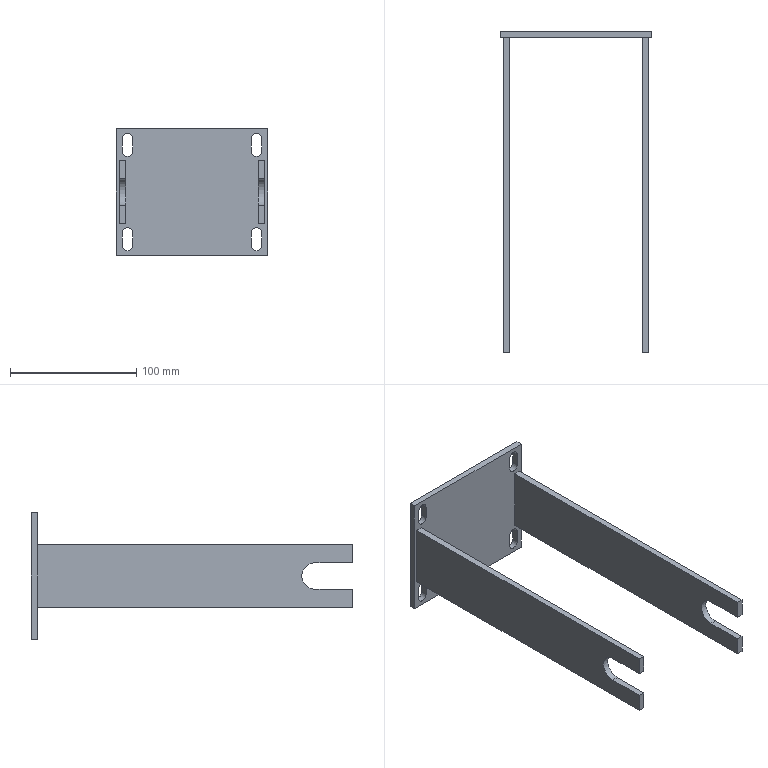Part | SolidWorks | features ICE 3, MirrorPattern 2, Extrusion 1 | 1 solid | 44 faces | box 120 x 255 x 100 mm | volume 174249 mm3 | plane 30 | cylinder 14 | commonest cylinder face diameters 8.258 x12 21 x2
STEP:
#1=CARTESIAN_POINT('',(111.116,0.,-3.551));
#2=VERTEX_POINT('',#1);
#3=CARTESIAN_POINT('',(115.245,0.,-7.68));
#4=VERTEX_POINT('',#3);
#5=CARTESIAN_POINT('',(111.116,0.,-7.68));
#6=DIRECTION('',(0.,1.,0.));
#7=DIRECTION('',(0.,0.,-1.));
#8=AXIS2_PLACEMENT_3D('',#5,#6,#7);
#9=CIRCLE('',#8,4.129);
#10=EDGE_CURVE('',#2,#4,#9,.T.);
#11=ORIENTED_EDGE('',*,*,#10,.F.);
#12=CARTESIAN_POINT('',(111.116,5.,-3.551));
#13=VERTEX_POINT('',#12);
#14=CARTESIAN_POINT('',(111.116,0.,-3.551));
#15=DIRECTION('',(0.,1.,0.));
#16=VECTOR('',#15,1000.);
#17=LINE('',#14,#16);
#18=EDGE_CURVE('',#2,#13,#17,.T.);
#19=ORIENTED_EDGE('',*,*,#18,.T.);
#20=CARTESIAN_POINT('',(115.245,5.,-7.68));
#21=VERTEX_POINT('',#20);
#22=CARTESIAN_POINT('',(111.116,5.,-7.68));
#23=DIRECTION('',(0.,1.,0.));
#24=DIRECTION('',(0.,0.,-1.));
#25=AXIS2_PLACEMENT_3D('',#22,#23,#24);
#26=CIRCLE('',#25,4.129);
#27=EDGE_CURVE('',#13,#21,#26,.T.);
#28=ORIENTED_EDGE('',*,*,#27,.T.);
#29=CARTESIAN_POINT('',(115.245,0.,-7.68));
#30=DIRECTION('',(0.,1.,0.));
#31=VECTOR('',#30,1000.);
#32=LINE('',#29,#31);
#33=EDGE_CURVE('',#4,#21,#32,.T.);
#34=ORIENTED_EDGE('',*,*,#33,.F.);
#35=EDGE_LOOP('',(#11,#19,#28,#34));
#36=FACE_OUTER_BOUND('',#35,.T.);
#37=CARTESIAN_POINT('',(111.116,0.,-7.68));
#38=DIRECTION('',(0.,1.,0.));
#39=DIRECTION('',(0.,0.,1.));
#40=AXIS2_PLACEMENT_3D('',#37,#38,#39);
#41=CYLINDRICAL_SURFACE('',#40,4.129);
#42=ADVANCED_FACE('',(#36),#41,.F.);
#43=CARTESIAN_POINT('',(13.013,0.,-7.68));
#44=VERTEX_POINT('',#43);
#45=CARTESIAN_POINT('',(8.884,0.,-3.551));
#46=VERTEX_POINT('',#45);
#47=CARTESIAN_POINT('',(8.884,0.,-7.68));
#48=DIRECTION('',(0.,-1.,0.));
#49=DIRECTION('',(0.,0.,-1.));
#50=AXIS2_PLACEMENT_3D('',#47,#48,#49);
#51=CIRCLE('',#50,4.129);
#52=EDGE_CURVE('',#44,#46,#51,.T.);
#53=ORIENTED_EDGE('',*,*,#52,.T.);
#54=CARTESIAN_POINT('',(8.884,5.,-3.551));
#55=VERTEX_POINT('',#54);
#56=CARTESIAN_POINT('',(8.884,0.,-3.551));
#57=DIRECTION('',(0.,1.,0.));
#58=VECTOR('',#57,1000.);
#59=LINE('',#56,#58);
#60=EDGE_CURVE('',#46,#55,#59,.T.);
#61=ORIENTED_EDGE('',*,*,#60,.T.);
#62=CARTESIAN_POINT('',(13.013,5.,-7.68));
#63=VERTEX_POINT('',#62);
#64=CARTESIAN_POINT('',(8.884,5.,-7.68));
#65=DIRECTION('',(0.,-1.,0.));
#66=DIRECTION('',(0.,0.,-1.));
#67=AXIS2_PLACEMENT_3D('',#64,#65,#66);
#68=CIRCLE('',#67,4.129);
#69=EDGE_CURVE('',#63,#55,#68,.T.);
#70=ORIENTED_EDGE('',*,*,#69,.F.);
#71=CARTESIAN_POINT('',(13.013,0.,-7.68));
#72=DIRECTION('',(0.,1.,0.));
#73=VECTOR('',#72,1000.);
#74=LINE('',#71,#73);
#75=EDGE_CURVE('',#44,#63,#74,.T.);
#76=ORIENTED_EDGE('',*,*,#75,.F.);
#77=EDGE_LOOP('',(#53,#61,#70,#76));
#78=FACE_OUTER_BOUND('',#77,.T.);
#79=CARTESIAN_POINT('',(8.884,0.,-7.68));
#80=DIRECTION('',(0.,1.,0.));
#81=DIRECTION('',(0.,0.,1.));
#82=AXIS2_PLACEMENT_3D('',#79,#80,#81);
#83=CYLINDRICAL_SURFACE('',#82,4.129);
#84=ADVANCED_FACE('',(#78),#83,.F.);
#85=CARTESIAN_POINT('',(115.245,0.,-82.342));
#86=VERTEX_POINT('',#85);
#87=CARTESIAN_POINT('',(111.116,0.,-78.214));
#88=VERTEX_POINT('',#87);
#89=CARTESIAN_POINT('',(111.116,0.,-82.342));
#90=DIRECTION('',(0.,-1.,0.));
#91=DIRECTION('',(0.,0.,1.));
#92=AXIS2_PLACEMENT_3D('',#89,#90,#91);
#93=CIRCLE('',#92,4.129);
#94=EDGE_CURVE('',#86,#88,#93,.T.);
#95=ORIENTED_EDGE('',*,*,#94,.T.);
#96=CARTESIAN_POINT('',(111.116,5.,-78.214));
#97=VERTEX_POINT('',#96);
#98=CARTESIAN_POINT('',(111.116,0.,-78.214));
#99=DIRECTION('',(0.,1.,0.));
#100=VECTOR('',#99,1000.);
#101=LINE('',#98,#100);
#102=EDGE_CURVE('',#88,#97,#101,.T.);
#103=ORIENTED_EDGE('',*,*,#102,.T.);
#104=CARTESIAN_POINT('',(115.245,5.,-82.342));
#105=VERTEX_POINT('',#104);
#106=CARTESIAN_POINT('',(111.116,5.,-82.342));
#107=DIRECTION('',(0.,-1.,0.));
#108=DIRECTION('',(0.,0.,1.));
#109=AXIS2_PLACEMENT_3D('',#106,#107,#108);
#110=CIRCLE('',#109,4.129);
#111=EDGE_CURVE('',#105,#97,#110,.T.);
#112=ORIENTED_EDGE('',*,*,#111,.F.);
#113=CARTESIAN_POINT('',(115.245,0.,-82.342));
#114=DIRECTION('',(0.,1.,0.));
#115=VECTOR('',#114,1000.);
#116=LINE('',#113,#115);
#117=EDGE_CURVE('',#86,#105,#116,.T.);
#118=ORIENTED_EDGE('',*,*,#117,.F.);
#119=EDGE_LOOP('',(#95,#103,#112,#118));
#120=FACE_OUTER_BOUND('',#119,.T.);
#121=CARTESIAN_POINT('',(111.116,0.,-82.342));
#122=DIRECTION('',(0.,1.,0.));
#123=DIRECTION('',(0.,0.,1.));
#124=AXIS2_PLACEMENT_3D('',#121,#122,#123);
#125=CYLINDRICAL_SURFACE('',#124,4.129);
#126=ADVANCED_FACE('',(#120),#125,.F.);
#127=CARTESIAN_POINT('',(8.884,0.,-78.214));
#128=VERTEX_POINT('',#127);
#129=CARTESIAN_POINT('',(13.013,0.,-82.342));
#130=VERTEX_POINT('',#129);
#131=CARTESIAN_POINT('',(8.884,0.,-82.342));
#132=DIRECTION('',(0.,1.,0.));
#133=DIRECTION('',(0.,0.,1.));
#134=AXIS2_PLACEMENT_3D('',#131,#132,#133);
#135=CIRCLE('',#134,4.129);
#136=EDGE_CURVE('',#128,#130,#135,.T.);
#137=ORIENTED_EDGE('',*,*,#136,.F.);
#138=CARTESIAN_POINT('',(8.884,5.,-78.214));
#139=VERTEX_POINT('',#138);
#140=CARTESIAN_POINT('',(8.884,0.,-78.214));
#141=DIRECTION('',(0.,1.,0.));
#142=VECTOR('',#141,1000.);
#143=LINE('',#140,#142);
#144=EDGE_CURVE('',#128,#139,#143,.T.);
#145=ORIENTED_EDGE('',*,*,#144,.T.);
#146=CARTESIAN_POINT('',(13.013,5.,-82.342));
#147=VERTEX_POINT('',#146);
#148=CARTESIAN_POINT('',(8.884,5.,-82.342));
#149=DIRECTION('',(0.,1.,0.));
#150=DIRECTION('',(0.,0.,1.));
#151=AXIS2_PLACEMENT_3D('',#148,#149,#150);
#152=CIRCLE('',#151,4.129);
#153=EDGE_CURVE('',#139,#147,#152,.T.);
#154=ORIENTED_EDGE('',*,*,#153,.T.);
#155=CARTESIAN_POINT('',(13.013,0.,-82.342));
#156=DIRECTION('',(0.,1.,0.));
#157=VECTOR('',#156,1000.);
#158=LINE('',#155,#157);
#159=EDGE_CURVE('',#130,#147,#158,.T.);
#160=ORIENTED_EDGE('',*,*,#159,.F.);
#161=EDGE_LOOP('',(#137,#145,#154,#160));
#162=FACE_OUTER_BOUND('',#161,.T.);
#163=CARTESIAN_POINT('',(8.884,0.,-82.342));
#164=DIRECTION('',(0.,1.,0.));
#165=DIRECTION('',(0.,0.,1.));
#166=AXIS2_PLACEMENT_3D('',#163,#164,#165);
#167=CYLINDRICAL_SURFACE('',#166,4.129);
#168=ADVANCED_FACE('',(#162),#167,.F.);
#169=CARTESIAN_POINT('',(117.5,-250.,-60.5));
#170=VERTEX_POINT('',#169);
#171=CARTESIAN_POINT('',(112.5,-250.,-60.5));
#172=VERTEX_POINT('',#171);
#173=CARTESIAN_POINT('',(452.5,-250.,-60.5));
#174=DIRECTION('',(-1.,0.,0.));
#175=VECTOR('',#174,1000.);
#176=LINE('',#173,#175);
#177=EDGE_CURVE('',#170,#172,#176,.T.);
#178=ORIENTED_EDGE('',*,*,#177,.T.);
#179=CARTESIAN_POINT('',(112.5,-250.,-75.));
#180=VERTEX_POINT('',#179);
#181=CARTESIAN_POINT('',(112.5,-250.,-45.));
#182=DIRECTION('',(0.,0.,-1.));
#183=VECTOR('',#182,1000.);
#184=LINE('',#181,#183);
#185=EDGE_CURVE('',#172,#180,#184,.T.);
#186=ORIENTED_EDGE('',*,*,#185,.T.);
#187=CARTESIAN_POINT('',(117.5,-250.,-75.));
#188=VERTEX_POINT('',#187);
#189=CARTESIAN_POINT('',(112.5,-250.,-75.));
#190=DIRECTION('',(1.,0.,0.));
#191=VECTOR('',#190,1000.);
#192=LINE('',#189,#191);
#193=EDGE_CURVE('',#180,#188,#192,.T.);
#194=ORIENTED_EDGE('',*,*,#193,.T.);
#195=CARTESIAN_POINT('',(117.5,-250.,-45.));
#196=DIRECTION('',(0.,0.,1.));
#197=VECTOR('',#196,1000.);
#198=LINE('',#195,#197);
#199=EDGE_CURVE('',#188,#170,#198,.T.);
#200=ORIENTED_EDGE('',*,*,#199,.T.);
#201=EDGE_LOOP('',(#178,#186,#194,#200));
#202=FACE_OUTER_BOUND('',#201,.T.);
#203=CARTESIAN_POINT('',(0.,-250.,0.));
#204=DIRECTION('',(0.,-1.,0.));
#205=DIRECTION('',(0.,0.,-1.));
#206=AXIS2_PLACEMENT_3D('',#203,#204,#205);
#207=PLANE('',#206);
#208=ADVANCED_FACE('',(#202),#207,.T.);
#209=CARTESIAN_POINT('',(7.5,-250.,-75.));
#210=VERTEX_POINT('',#209);
#211=CARTESIAN_POINT('',(7.5,-250.,-60.5));
#212=VERTEX_POINT('',#211);
#213=CARTESIAN_POINT('',(7.5,-250.,-50.));
#214=DIRECTION('',(0.,0.,1.));
#215=VECTOR('',#214,1000.);
#216=LINE('',#213,#215);
#217=EDGE_CURVE('',#210,#212,#216,.T.);
#218=ORIENTED_EDGE('',*,*,#217,.T.);
#219=CARTESIAN_POINT('',(2.5,-250.,-60.5));
#220=VERTEX_POINT('',#219);
#221=CARTESIAN_POINT('',(0.,-250.,-60.5));
#222=DIRECTION('',(-1.,0.,0.));
#223=VECTOR('',#222,1000.);
#224=LINE('',#221,#223);
#225=EDGE_CURVE('',#212,#220,#224,.T.);
#226=ORIENTED_EDGE('',*,*,#225,.T.);
#227=CARTESIAN_POINT('',(2.5,-250.,-75.));
#228=VERTEX_POINT('',#227);
#229=CARTESIAN_POINT('',(2.5,-250.,-50.));
#230=DIRECTION('',(0.,0.,-1.));
#231=VECTOR('',#230,1000.);
#232=LINE('',#229,#231);
#233=EDGE_CURVE('',#220,#228,#232,.T.);
#234=ORIENTED_EDGE('',*,*,#233,.T.);
#235=CARTESIAN_POINT('',(7.5,-250.,-75.));
#236=DIRECTION('',(1.,0.,0.));
#237=VECTOR('',#236,1000.);
#238=LINE('',#235,#237);
#239=EDGE_CURVE('',#228,#210,#238,.T.);
#240=ORIENTED_EDGE('',*,*,#239,.T.);
#241=EDGE_LOOP('',(#218,#226,#234,#240));
#242=FACE_OUTER_BOUND('',#241,.T.);
#243=CARTESIAN_POINT('',(0.,-250.,0.));
#244=DIRECTION('',(0.,1.,0.));
#245=DIRECTION('',(0.,0.,1.));
#246=AXIS2_PLACEMENT_3D('',#243,#244,#245);
#247=PLANE('',#246);
#248=ADVANCED_FACE('',(#242),#247,.F.);
#249=CARTESIAN_POINT('',(112.5,0.,-75.));
#250=VERTEX_POINT('',#249);
#251=CARTESIAN_POINT('',(117.5,0.,-75.));
#252=VERTEX_POINT('',#251);
#253=CARTESIAN_POINT('',(112.5,0.,-75.));
#254=DIRECTION('',(1.,0.,0.));
#255=VECTOR('',#254,1000.);
#256=LINE('',#253,#255);
#257=EDGE_CURVE('',#250,#252,#256,.T.);
#258=ORIENTED_EDGE('',*,*,#257,.F.);
#259=CARTESIAN_POINT('',(112.5,0.,-25.));
#260=VERTEX_POINT('',#259);
#261=CARTESIAN_POINT('',(112.5,0.,-45.));
#262=DIRECTION('',(0.,0.,-1.));
#263=VECTOR('',#262,1000.);
#264=LINE('',#261,#263);
#265=EDGE_CURVE('',#260,#250,#264,.T.);
#266=ORIENTED_EDGE('',*,*,#265,.F.);
#267=CARTESIAN_POINT('',(117.5,0.,-25.));
#268=VERTEX_POINT('',#267);
#269=CARTESIAN_POINT('',(117.5,0.,-25.));
#270=DIRECTION('',(-1.,0.,0.));
#271=VECTOR('',#270,1000.);
#272=LINE('',#269,#271);
#273=EDGE_CURVE('',#268,#260,#272,.T.);
#274=ORIENTED_EDGE('',*,*,#273,.F.);
#275=CARTESIAN_POINT('',(117.5,0.,-45.));
#276=DIRECTION('',(0.,0.,1.));
#277=VECTOR('',#276,1000.);
#278=LINE('',#275,#277);
#279=EDGE_CURVE('',#252,#268,#278,.T.);
#280=ORIENTED_EDGE('',*,*,#279,.F.);
#281=EDGE_LOOP('',(#258,#266,#274,#280));
#282=FACE_BOUND('',#281,.T.);
#283=CARTESIAN_POINT('',(106.987,0.,-7.68));
#284=VERTEX_POINT('',#283);
#285=CARTESIAN_POINT('',(111.116,0.,-7.68));
#286=DIRECTION('',(0.,1.,0.));
#287=DIRECTION('',(0.,0.,-1.));
#288=AXIS2_PLACEMENT_3D('',#285,#286,#287);
#289=CIRCLE('',#288,4.129);
#290=EDGE_CURVE('',#284,#2,#289,.T.);
#291=ORIENTED_EDGE('',*,*,#290,.T.);
#292=ORIENTED_EDGE('',*,*,#10,.T.);
#293=CARTESIAN_POINT('',(115.245,0.,-17.658));
#294=VERTEX_POINT('',#293);
#295=CARTESIAN_POINT('',(115.245,0.,-7.68));
#296=DIRECTION('',(0.,0.,-1.));
#297=VECTOR('',#296,1000.);
#298=LINE('',#295,#297);
#299=EDGE_CURVE('',#4,#294,#298,.T.);
#300=ORIENTED_EDGE('',*,*,#299,.T.);
#301=CARTESIAN_POINT('',(106.987,0.,-17.658));
#302=VERTEX_POINT('',#301);
#303=CARTESIAN_POINT('',(111.116,0.,-17.658));
#304=DIRECTION('',(0.,1.,0.));
#305=DIRECTION('',(0.,0.,-1.));
#306=AXIS2_PLACEMENT_3D('',#303,#304,#305);
#307=CIRCLE('',#306,4.129);
#308=EDGE_CURVE('',#294,#302,#307,.T.);
#309=ORIENTED_EDGE('',*,*,#308,.T.);
#310=CARTESIAN_POINT('',(106.987,0.,-7.68));
#311=DIRECTION('',(0.,0.,1.));
#312=VECTOR('',#311,1000.);
#313=LINE('',#310,#312);
#314=EDGE_CURVE('',#302,#284,#313,.T.);
#315=ORIENTED_EDGE('',*,*,#314,.T.);
#316=EDGE_LOOP('',(#291,#292,#300,#309,#315));
#317=FACE_BOUND('',#316,.T.);
#318=CARTESIAN_POINT('',(115.245,0.,-92.32));
#319=VERTEX_POINT('',#318);
#320=CARTESIAN_POINT('',(115.245,0.,-92.32));
#321=DIRECTION('',(0.,0.,1.));
#322=VECTOR('',#321,1000.);
#323=LINE('',#320,#322);
#324=EDGE_CURVE('',#319,#86,#323,.T.);
#325=ORIENTED_EDGE('',*,*,#324,.F.);
#326=CARTESIAN_POINT('',(106.987,0.,-92.32));
#327=VERTEX_POINT('',#326);
#328=CARTESIAN_POINT('',(111.116,0.,-92.32));
#329=DIRECTION('',(0.,-1.,0.));
#330=DIRECTION('',(0.,0.,1.));
#331=AXIS2_PLACEMENT_3D('',#328,#329,#330);
#332=CIRCLE('',#331,4.129);
#333=EDGE_CURVE('',#327,#319,#332,.T.);
#334=ORIENTED_EDGE('',*,*,#333,.F.);
#335=CARTESIAN_POINT('',(106.987,0.,-82.342));
#336=VERTEX_POINT('',#335);
#337=CARTESIAN_POINT('',(106.987,0.,-92.32));
#338=DIRECTION('',(0.,0.,-1.));
#339=VECTOR('',#338,1000.);
#340=LINE('',#337,#339);
#341=EDGE_CURVE('',#336,#327,#340,.T.);
#342=ORIENTED_EDGE('',*,*,#341,.F.);
#343=CARTESIAN_POINT('',(111.116,0.,-82.342));
#344=DIRECTION('',(0.,-1.,0.));
#345=DIRECTION('',(0.,0.,1.));
#346=AXIS2_PLACEMENT_3D('',#343,#344,#345);
#347=CIRCLE('',#346,4.129);
#348=EDGE_CURVE('',#88,#336,#347,.T.);
#349=ORIENTED_EDGE('',*,*,#348,.F.);
#350=ORIENTED_EDGE('',*,*,#94,.F.);
#351=EDGE_LOOP('',(#325,#334,#342,#349,#350));
#352=FACE_BOUND('',#351,.T.);
#353=CARTESIAN_POINT('',(13.013,0.,-92.32));
#354=VERTEX_POINT('',#353);
#355=CARTESIAN_POINT('',(4.755,0.,-92.32));
#356=VERTEX_POINT('',#355);
#357=CARTESIAN_POINT('',(8.884,0.,-92.32));
#358=DIRECTION('',(0.,1.,0.));
#359=DIRECTION('',(0.,0.,1.));
#360=AXIS2_PLACEMENT_3D('',#357,#358,#359);
#361=CIRCLE('',#360,4.129);
#362=EDGE_CURVE('',#354,#356,#361,.T.);
#363=ORIENTED_EDGE('',*,*,#362,.T.);
#364=CARTESIAN_POINT('',(4.755,0.,-82.342));
#365=VERTEX_POINT('',#364);
#366=CARTESIAN_POINT('',(4.755,0.,-92.32));
#367=DIRECTION('',(0.,0.,1.));
#368=VECTOR('',#367,1000.);
#369=LINE('',#366,#368);
#370=EDGE_CURVE('',#356,#365,#369,.T.);
#371=ORIENTED_EDGE('',*,*,#370,.T.);
#372=CARTESIAN_POINT('',(8.884,0.,-82.342));
#373=DIRECTION('',(0.,1.,0.));
#374=DIRECTION('',(0.,0.,1.));
#375=AXIS2_PLACEMENT_3D('',#372,#373,#374);
#376=CIRCLE('',#375,4.129);
#377=EDGE_CURVE('',#365,#128,#376,.T.);
#378=ORIENTED_EDGE('',*,*,#377,.T.);
#379=ORIENTED_EDGE('',*,*,#136,.T.);
#380=CARTESIAN_POINT('',(13.013,0.,-92.32));
#381=DIRECTION('',(0.,0.,-1.));
#382=VECTOR('',#381,1000.);
#383=LINE('',#380,#382);
#384=EDGE_CURVE('',#130,#354,#383,.T.);
#385=ORIENTED_EDGE('',*,*,#384,.T.);
#386=EDGE_LOOP('',(#363,#371,#378,#379,#385));
#387=FACE_BOUND('',#386,.T.);
#388=CARTESIAN_POINT('',(0.,0.,-100.));
#389=VERTEX_POINT('',#388);
#390=CARTESIAN_POINT('',(0.,0.,0.));
#391=VERTEX_POINT('',#390);
#392=CARTESIAN_POINT('',(0.,0.,0.));
#393=DIRECTION('',(0.,0.,1.));
#394=VECTOR('',#393,1000.);
#395=LINE('',#392,#394);
#396=EDGE_CURVE('',#389,#391,#395,.T.);
#397=ORIENTED_EDGE('',*,*,#396,.F.);
#398=CARTESIAN_POINT('',(120.,0.,-100.));
#399=VERTEX_POINT('',#398);
#400=CARTESIAN_POINT('',(0.,0.,-100.));
#401=DIRECTION('',(-1.,0.,0.));
#402=VECTOR('',#401,1000.);
#403=LINE('',#400,#402);
#404=EDGE_CURVE('',#399,#389,#403,.T.);
#405=ORIENTED_EDGE('',*,*,#404,.F.);
#406=CARTESIAN_POINT('',(120.,0.,0.));
#407=VERTEX_POINT('',#406);
#408=CARTESIAN_POINT('',(120.,0.,0.));
#409=DIRECTION('',(0.,0.,-1.));
#410=VECTOR('',#409,1000.);
#411=LINE('',#408,#410);
#412=EDGE_CURVE('',#407,#399,#411,.T.);
#413=ORIENTED_EDGE('',*,*,#412,.F.);
#414=CARTESIAN_POINT('',(0.,0.,0.));
#415=DIRECTION('',(1.,0.,0.));
#416=VECTOR('',#415,1000.);
#417=LINE('',#414,#416);
#418=EDGE_CURVE('',#391,#407,#417,.T.);
#419=ORIENTED_EDGE('',*,*,#418,.F.);
#420=EDGE_LOOP('',(#397,#405,#413,#419));
#421=FACE_OUTER_BOUND('',#420,.T.);
#422=CARTESIAN_POINT('',(4.755,0.,-7.68));
#423=VERTEX_POINT('',#422);
#424=CARTESIAN_POINT('',(4.755,0.,-17.658));
#425=VERTEX_POINT('',#424);
#426=CARTESIAN_POINT('',(4.755,0.,-7.68));
#427=DIRECTION('',(0.,0.,-1.));
#428=VECTOR('',#427,1000.);
#429=LINE('',#426,#428);
#430=EDGE_CURVE('',#423,#425,#429,.T.);
#431=ORIENTED_EDGE('',*,*,#430,.F.);
#432=CARTESIAN_POINT('',(8.884,0.,-7.68));
#433=DIRECTION('',(0.,-1.,0.));
#434=DIRECTION('',(0.,0.,-1.));
#435=AXIS2_PLACEMENT_3D('',#432,#433,#434);
#436=CIRCLE('',#435,4.129);
#437=EDGE_CURVE('',#46,#423,#436,.T.);
#438=ORIENTED_EDGE('',*,*,#437,.F.);
#439=ORIENTED_EDGE('',*,*,#52,.F.);
#440=CARTESIAN_POINT('',(13.013,0.,-17.658));
#441=VERTEX_POINT('',#440);
#442=CARTESIAN_POINT('',(13.013,0.,-7.68));
#443=DIRECTION('',(0.,0.,1.));
#444=VECTOR('',#443,1000.);
#445=LINE('',#442,#444);
#446=EDGE_CURVE('',#441,#44,#445,.T.);
#447=ORIENTED_EDGE('',*,*,#446,.F.);
#448=CARTESIAN_POINT('',(8.884,0.,-17.658));
#449=DIRECTION('',(0.,-1.,0.));
#450=DIRECTION('',(0.,0.,-1.));
#451=AXIS2_PLACEMENT_3D('',#448,#449,#450);
#452=CIRCLE('',#451,4.129);
#453=EDGE_CURVE('',#425,#441,#452,.T.);
#454=ORIENTED_EDGE('',*,*,#453,.F.);
#455=EDGE_LOOP('',(#431,#438,#439,#447,#454));
#456=FACE_BOUND('',#455,.T.);
#457=CARTESIAN_POINT('',(2.5,0.,-75.));
#458=VERTEX_POINT('',#457);
#459=CARTESIAN_POINT('',(7.5,0.,-75.));
#460=VERTEX_POINT('',#459);
#461=CARTESIAN_POINT('',(7.5,0.,-75.));
#462=DIRECTION('',(1.,0.,0.));
#463=VECTOR('',#462,1000.);
#464=LINE('',#461,#463);
#465=EDGE_CURVE('',#458,#460,#464,.T.);
#466=ORIENTED_EDGE('',*,*,#465,.F.);
#467=CARTESIAN_POINT('',(2.5,0.,-25.));
#468=VERTEX_POINT('',#467);
#469=CARTESIAN_POINT('',(2.5,0.,-50.));
#470=DIRECTION('',(0.,0.,-1.));
#471=VECTOR('',#470,1000.);
#472=LINE('',#469,#471);
#473=EDGE_CURVE('',#468,#458,#472,.T.);
#474=ORIENTED_EDGE('',*,*,#473,.F.);
#475=CARTESIAN_POINT('',(7.5,0.,-25.));
#476=VERTEX_POINT('',#475);
#477=CARTESIAN_POINT('',(2.5,0.,-25.));
#478=DIRECTION('',(-1.,0.,0.));
#479=VECTOR('',#478,1000.);
#480=LINE('',#477,#479);
#481=EDGE_CURVE('',#476,#468,#480,.T.);
#482=ORIENTED_EDGE('',*,*,#481,.F.);
#483=CARTESIAN_POINT('',(7.5,0.,-50.));
#484=DIRECTION('',(0.,0.,1.));
#485=VECTOR('',#484,1000.);
#486=LINE('',#483,#485);
#487=EDGE_CURVE('',#460,#476,#486,.T.);
#488=ORIENTED_EDGE('',*,*,#487,.F.);
#489=EDGE_LOOP('',(#466,#474,#482,#488));
#490=FACE_BOUND('',#489,.T.);
#491=CARTESIAN_POINT('',(0.,0.,0.));
#492=DIRECTION('',(0.,-1.,0.));
#493=DIRECTION('',(0.,0.,-1.));
#494=AXIS2_PLACEMENT_3D('',#491,#492,#493);
#495=PLANE('',#494);
#496=ADVANCED_FACE('',(#282,#317,#352,#387,#421,#456,#490),#495,.T.);
#497=CARTESIAN_POINT('',(115.245,5.,-17.658));
#498=VERTEX_POINT('',#497);
#499=CARTESIAN_POINT('',(115.245,5.,-7.68));
#500=DIRECTION('',(0.,0.,-1.));
#501=VECTOR('',#500,1000.);
#502=LINE('',#499,#501);
#503=EDGE_CURVE('',#21,#498,#502,.T.);
#504=ORIENTED_EDGE('',*,*,#503,.F.);
#505=ORIENTED_EDGE('',*,*,#27,.F.);
#506=CARTESIAN_POINT('',(106.987,5.,-7.68));
#507=VERTEX_POINT('',#506);
#508=CARTESIAN_POINT('',(111.116,5.,-7.68));
#509=DIRECTION('',(0.,1.,0.));
#510=DIRECTION('',(0.,0.,-1.));
#511=AXIS2_PLACEMENT_3D('',#508,#509,#510);
#512=CIRCLE('',#511,4.129);
#513=EDGE_CURVE('',#507,#13,#512,.T.);
#514=ORIENTED_EDGE('',*,*,#513,.F.);
#515=CARTESIAN_POINT('',(106.987,5.,-17.658));
#516=VERTEX_POINT('',#515);
#517=CARTESIAN_POINT('',(106.987,5.,-7.68));
#518=DIRECTION('',(0.,0.,1.));
#519=VECTOR('',#518,1000.);
#520=LINE('',#517,#519);
#521=EDGE_CURVE('',#516,#507,#520,.T.);
#522=ORIENTED_EDGE('',*,*,#521,.F.);
#523=CARTESIAN_POINT('',(111.116,5.,-17.658));
#524=DIRECTION('',(0.,1.,0.));
#525=DIRECTION('',(0.,0.,-1.));
#526=AXIS2_PLACEMENT_3D('',#523,#524,#525);
#527=CIRCLE('',#526,4.129);
#528=EDGE_CURVE('',#498,#516,#527,.T.);
#529=ORIENTED_EDGE('',*,*,#528,.F.);
#530=EDGE_LOOP('',(#504,#505,#514,#522,#529));
#531=FACE_BOUND('',#530,.T.);
#532=CARTESIAN_POINT('',(106.987,5.,-92.32));
#533=VERTEX_POINT('',#532);
#534=CARTESIAN_POINT('',(115.245,5.,-92.32));
#535=VERTEX_POINT('',#534);
#536=CARTESIAN_POINT('',(111.116,5.,-92.32));
#537=DIRECTION('',(0.,-1.,0.));
#538=DIRECTION('',(0.,0.,1.));
#539=AXIS2_PLACEMENT_3D('',#536,#537,#538);
#540=CIRCLE('',#539,4.129);
#541=EDGE_CURVE('',#533,#535,#540,.T.);
#542=ORIENTED_EDGE('',*,*,#541,.T.);
#543=CARTESIAN_POINT('',(115.245,5.,-92.32));
#544=DIRECTION('',(0.,0.,1.));
#545=VECTOR('',#544,1000.);
#546=LINE('',#543,#545);
#547=EDGE_CURVE('',#535,#105,#546,.T.);
#548=ORIENTED_EDGE('',*,*,#547,.T.);
#549=ORIENTED_EDGE('',*,*,#111,.T.);
#550=CARTESIAN_POINT('',(106.987,5.,-82.342));
#551=VERTEX_POINT('',#550);
#552=CARTESIAN_POINT('',(111.116,5.,-82.342));
#553=DIRECTION('',(0.,-1.,0.));
#554=DIRECTION('',(0.,0.,1.));
#555=AXIS2_PLACEMENT_3D('',#552,#553,#554);
#556=CIRCLE('',#555,4.129);
#557=EDGE_CURVE('',#97,#551,#556,.T.);
#558=ORIENTED_EDGE('',*,*,#557,.T.);
#559=CARTESIAN_POINT('',(106.987,5.,-92.32));
#560=DIRECTION('',(0.,0.,-1.));
#561=VECTOR('',#560,1000.);
#562=LINE('',#559,#561);
#563=EDGE_CURVE('',#551,#533,#562,.T.);
#564=ORIENTED_EDGE('',*,*,#563,.T.);
#565=EDGE_LOOP('',(#542,#548,#549,#558,#564));
#566=FACE_BOUND('',#565,.T.);
#567=CARTESIAN_POINT('',(4.755,5.,-92.32));
#568=VERTEX_POINT('',#567);
#569=CARTESIAN_POINT('',(4.755,5.,-82.342));
#570=VERTEX_POINT('',#569);
#571=CARTESIAN_POINT('',(4.755,5.,-92.32));
#572=DIRECTION('',(0.,0.,1.));
#573=VECTOR('',#572,1000.);
#574=LINE('',#571,#573);
#575=EDGE_CURVE('',#568,#570,#574,.T.);
#576=ORIENTED_EDGE('',*,*,#575,.F.);
#577=CARTESIAN_POINT('',(13.013,5.,-92.32));
#578=VERTEX_POINT('',#577);
#579=CARTESIAN_POINT('',(8.884,5.,-92.32));
#580=DIRECTION('',(0.,1.,0.));
#581=DIRECTION('',(0.,0.,1.));
#582=AXIS2_PLACEMENT_3D('',#579,#580,#581);
#583=CIRCLE('',#582,4.129);
#584=EDGE_CURVE('',#578,#568,#583,.T.);
#585=ORIENTED_EDGE('',*,*,#584,.F.);
#586=CARTESIAN_POINT('',(13.013,5.,-92.32));
#587=DIRECTION('',(0.,0.,-1.));
#588=VECTOR('',#587,1000.);
#589=LINE('',#586,#588);
#590=EDGE_CURVE('',#147,#578,#589,.T.);
#591=ORIENTED_EDGE('',*,*,#590,.F.);
#592=ORIENTED_EDGE('',*,*,#153,.F.);
#593=CARTESIAN_POINT('',(8.884,5.,-82.342));
#594=DIRECTION('',(0.,1.,0.));
#595=DIRECTION('',(0.,0.,1.));
#596=AXIS2_PLACEMENT_3D('',#593,#594,#595);
#597=CIRCLE('',#596,4.129);
#598=EDGE_CURVE('',#570,#139,#597,.T.);
#599=ORIENTED_EDGE('',*,*,#598,.F.);
#600=EDGE_LOOP('',(#576,#585,#591,#592,#599));
#601=FACE_BOUND('',#600,.T.);
#602=CARTESIAN_POINT('',(0.,5.,-100.));
#603=VERTEX_POINT('',#602);
#604=CARTESIAN_POINT('',(0.,5.,0.));
#605=VERTEX_POINT('',#604);
#606=CARTESIAN_POINT('',(0.,5.,0.));
#607=DIRECTION('',(0.,0.,1.));
#608=VECTOR('',#607,1000.);
#609=LINE('',#606,#608);
#610=EDGE_CURVE('',#603,#605,#609,.T.);
#611=ORIENTED_EDGE('',*,*,#610,.T.);
#612=CARTESIAN_POINT('',(120.,5.,0.));
#613=VERTEX_POINT('',#612);
#614=CARTESIAN_POINT('',(0.,5.,0.));
#615=DIRECTION('',(1.,0.,0.));
#616=VECTOR('',#615,1000.);
#617=LINE('',#614,#616);
#618=EDGE_CURVE('',#605,#613,#617,.T.);
#619=ORIENTED_EDGE('',*,*,#618,.T.);
#620=CARTESIAN_POINT('',(120.,5.,-100.));
#621=VERTEX_POINT('',#620);
#622=CARTESIAN_POINT('',(120.,5.,0.));
#623=DIRECTION('',(0.,0.,-1.));
#624=VECTOR('',#623,1000.);
#625=LINE('',#622,#624);
#626=EDGE_CURVE('',#613,#621,#625,.T.);
#627=ORIENTED_EDGE('',*,*,#626,.T.);
#628=CARTESIAN_POINT('',(0.,5.,-100.));
#629=DIRECTION('',(-1.,0.,0.));
#630=VECTOR('',#629,1000.);
#631=LINE('',#628,#630);
#632=EDGE_CURVE('',#621,#603,#631,.T.);
#633=ORIENTED_EDGE('',*,*,#632,.T.);
#634=EDGE_LOOP('',(#611,#619,#627,#633));
#635=FACE_OUTER_BOUND('',#634,.T.);
#636=ORIENTED_EDGE('',*,*,#69,.T.);
#637=CARTESIAN_POINT('',(4.755,5.,-7.68));
#638=VERTEX_POINT('',#637);
#639=CARTESIAN_POINT('',(8.884,5.,-7.68));
#640=DIRECTION('',(0.,-1.,0.));
#641=DIRECTION('',(0.,0.,-1.));
#642=AXIS2_PLACEMENT_3D('',#639,#640,#641);
#643=CIRCLE('',#642,4.129);
#644=EDGE_CURVE('',#55,#638,#643,.T.);
#645=ORIENTED_EDGE('',*,*,#644,.T.);
#646=CARTESIAN_POINT('',(4.755,5.,-17.658));
#647=VERTEX_POINT('',#646);
#648=CARTESIAN_POINT('',(4.755,5.,-7.68));
#649=DIRECTION('',(0.,0.,-1.));
#650=VECTOR('',#649,1000.);
#651=LINE('',#648,#650);
#652=EDGE_CURVE('',#638,#647,#651,.T.);
#653=ORIENTED_EDGE('',*,*,#652,.T.);
#654=CARTESIAN_POINT('',(13.013,5.,-17.658));
#655=VERTEX_POINT('',#654);
#656=CARTESIAN_POINT('',(8.884,5.,-17.658));
#657=DIRECTION('',(0.,-1.,0.));
#658=DIRECTION('',(0.,0.,-1.));
#659=AXIS2_PLACEMENT_3D('',#656,#657,#658);
#660=CIRCLE('',#659,4.129);
#661=EDGE_CURVE('',#647,#655,#660,.T.);
#662=ORIENTED_EDGE('',*,*,#661,.T.);
#663=CARTESIAN_POINT('',(13.013,5.,-7.68));
#664=DIRECTION('',(0.,0.,1.));
#665=VECTOR('',#664,1000.);
#666=LINE('',#663,#665);
#667=EDGE_CURVE('',#655,#63,#666,.T.);
#668=ORIENTED_EDGE('',*,*,#667,.T.);
#669=EDGE_LOOP('',(#636,#645,#653,#662,#668));
#670=FACE_BOUND('',#669,.T.);
#671=CARTESIAN_POINT('',(0.,5.,0.));
#672=DIRECTION('',(0.,-1.,0.));
#673=DIRECTION('',(0.,0.,-1.));
#674=AXIS2_PLACEMENT_3D('',#671,#672,#673);
#675=PLANE('',#674);
#676=ADVANCED_FACE('',(#531,#566,#601,#635,#670),#675,.F.);
#677=ORIENTED_EDGE('',*,*,#396,.T.);
#678=CARTESIAN_POINT('',(0.,5.,0.));
#679=DIRECTION('',(0.,-1.,0.));
#680=VECTOR('',#679,1000.);
#681=LINE('',#678,#680);
#682=EDGE_CURVE('',#605,#391,#681,.T.);
#683=ORIENTED_EDGE('',*,*,#682,.F.);
#684=ORIENTED_EDGE('',*,*,#610,.F.);
#685=CARTESIAN_POINT('',(0.,5.,-100.));
#686=DIRECTION('',(0.,-1.,0.));
#687=VECTOR('',#686,1000.);
#688=LINE('',#685,#687);
#689=EDGE_CURVE('',#603,#389,#688,.T.);
#690=ORIENTED_EDGE('',*,*,#689,.T.);
#691=EDGE_LOOP('',(#677,#683,#684,#690));
#692=FACE_OUTER_BOUND('',#691,.T.);
#693=CARTESIAN_POINT('',(0.,5.,0.));
#694=DIRECTION('',(1.,0.,0.));
#695=DIRECTION('',(0.,0.,-1.));
#696=AXIS2_PLACEMENT_3D('',#693,#694,#695);
#697=PLANE('',#696);
#698=ADVANCED_FACE('',(#692),#697,.F.);
#699=ORIENTED_EDGE('',*,*,#418,.T.);
#700=CARTESIAN_POINT('',(120.,5.,0.));
#701=DIRECTION('',(0.,-1.,0.));
#702=VECTOR('',#701,1000.);
#703=LINE('',#700,#702);
#704=EDGE_CURVE('',#613,#407,#703,.T.);
#705=ORIENTED_EDGE('',*,*,#704,.F.);
#706=ORIENTED_EDGE('',*,*,#618,.F.);
#707=ORIENTED_EDGE('',*,*,#682,.T.);
#708=EDGE_LOOP('',(#699,#705,#706,#707));
#709=FACE_OUTER_BOUND('',#708,.T.);
#710=CARTESIAN_POINT('',(0.,5.,0.));
#711=DIRECTION('',(0.,0.,-1.));
#712=DIRECTION('',(-1.,0.,0.));
#713=AXIS2_PLACEMENT_3D('',#710,#711,#712);
#714=PLANE('',#713);
#715=ADVANCED_FACE('',(#709),#714,.F.);
#716=ORIENTED_EDGE('',*,*,#412,.T.);
#717=CARTESIAN_POINT('',(120.,5.,-100.));
#718=DIRECTION('',(0.,-1.,0.));
#719=VECTOR('',#718,1000.);
#720=LINE('',#717,#719);
#721=EDGE_CURVE('',#621,#399,#720,.T.);
#722=ORIENTED_EDGE('',*,*,#721,.F.);
#723=ORIENTED_EDGE('',*,*,#626,.F.);
#724=ORIENTED_EDGE('',*,*,#704,.T.);
#725=EDGE_LOOP('',(#716,#722,#723,#724));
#726=FACE_OUTER_BOUND('',#725,.T.);
#727=CARTESIAN_POINT('',(120.,5.,0.));
#728=DIRECTION('',(-1.,0.,0.));
#729=DIRECTION('',(0.,0.,1.));
#730=AXIS2_PLACEMENT_3D('',#727,#728,#729);
#731=PLANE('',#730);
#732=ADVANCED_FACE('',(#726),#731,.F.);
#733=ORIENTED_EDGE('',*,*,#404,.T.);
#734=ORIENTED_EDGE('',*,*,#689,.F.);
#735=ORIENTED_EDGE('',*,*,#632,.F.);
#736=ORIENTED_EDGE('',*,*,#721,.T.);
#737=EDGE_LOOP('',(#733,#734,#735,#736));
#738=FACE_OUTER_BOUND('',#737,.T.);
#739=CARTESIAN_POINT('',(0.,5.,-100.));
#740=DIRECTION('',(0.,0.,1.));
#741=DIRECTION('',(1.,0.,0.));
#742=AXIS2_PLACEMENT_3D('',#739,#740,#741);
#743=PLANE('',#742);
#744=ADVANCED_FACE('',(#738),#743,.F.);
#745=ORIENTED_EDGE('',*,*,#584,.T.);
#746=CARTESIAN_POINT('',(4.755,0.,-92.32));
#747=DIRECTION('',(0.,1.,0.));
#748=VECTOR('',#747,1000.);
#749=LINE('',#746,#748);
#750=EDGE_CURVE('',#356,#568,#749,.T.);
#751=ORIENTED_EDGE('',*,*,#750,.F.);
#752=ORIENTED_EDGE('',*,*,#362,.F.);
#753=CARTESIAN_POINT('',(13.013,0.,-92.32));
#754=DIRECTION('',(0.,1.,0.));
#755=VECTOR('',#754,1000.);
#756=LINE('',#753,#755);
#757=EDGE_CURVE('',#354,#578,#756,.T.);
#758=ORIENTED_EDGE('',*,*,#757,.T.);
#759=EDGE_LOOP('',(#745,#751,#752,#758));
#760=FACE_OUTER_BOUND('',#759,.T.);
#761=CARTESIAN_POINT('',(8.884,0.,-92.32));
#762=DIRECTION('',(0.,1.,0.));
#763=DIRECTION('',(0.,0.,1.));
#764=AXIS2_PLACEMENT_3D('',#761,#762,#763);
#765=CYLINDRICAL_SURFACE('',#764,4.129);
#766=ADVANCED_FACE('',(#760),#765,.F.);
#767=ORIENTED_EDGE('',*,*,#590,.T.);
#768=ORIENTED_EDGE('',*,*,#757,.F.);
#769=ORIENTED_EDGE('',*,*,#384,.F.);
#770=ORIENTED_EDGE('',*,*,#159,.T.);
#771=EDGE_LOOP('',(#767,#768,#769,#770));
#772=FACE_OUTER_BOUND('',#771,.T.);
#773=CARTESIAN_POINT('',(13.013,0.,-92.32));
#774=DIRECTION('',(1.,0.,0.));
#775=DIRECTION('',(0.,0.,-1.));
#776=AXIS2_PLACEMENT_3D('',#773,#774,#775);
#777=PLANE('',#776);
#778=ADVANCED_FACE('',(#772),#777,.F.);
#779=ORIENTED_EDGE('',*,*,#144,.F.);
#780=ORIENTED_EDGE('',*,*,#377,.F.);
#781=CARTESIAN_POINT('',(4.755,0.,-82.342));
#782=DIRECTION('',(0.,1.,0.));
#783=VECTOR('',#782,1000.);
#784=LINE('',#781,#783);
#785=EDGE_CURVE('',#365,#570,#784,.T.);
#786=ORIENTED_EDGE('',*,*,#785,.T.);
#787=ORIENTED_EDGE('',*,*,#598,.T.);
#788=EDGE_LOOP('',(#779,#780,#786,#787));
#789=FACE_OUTER_BOUND('',#788,.T.);
#790=CARTESIAN_POINT('',(8.884,0.,-82.342));
#791=DIRECTION('',(0.,1.,0.));
#792=DIRECTION('',(0.,0.,1.));
#793=AXIS2_PLACEMENT_3D('',#790,#791,#792);
#794=CYLINDRICAL_SURFACE('',#793,4.129);
#795=ADVANCED_FACE('',(#789),#794,.F.);
#796=ORIENTED_EDGE('',*,*,#575,.T.);
#797=ORIENTED_EDGE('',*,*,#785,.F.);
#798=ORIENTED_EDGE('',*,*,#370,.F.);
#799=ORIENTED_EDGE('',*,*,#750,.T.);
#800=EDGE_LOOP('',(#796,#797,#798,#799));
#801=FACE_OUTER_BOUND('',#800,.T.);
#802=CARTESIAN_POINT('',(4.755,0.,-92.32));
#803=DIRECTION('',(-1.,0.,0.));
#804=DIRECTION('',(0.,0.,1.));
#805=AXIS2_PLACEMENT_3D('',#802,#803,#804);
#806=PLANE('',#805);
#807=ADVANCED_FACE('',(#801),#806,.F.);
#808=ORIENTED_EDGE('',*,*,#541,.F.);
#809=CARTESIAN_POINT('',(106.987,0.,-92.32));
#810=DIRECTION('',(0.,1.,0.));
#811=VECTOR('',#810,1000.);
#812=LINE('',#809,#811);
#813=EDGE_CURVE('',#327,#533,#812,.T.);
#814=ORIENTED_EDGE('',*,*,#813,.F.);
#815=ORIENTED_EDGE('',*,*,#333,.T.);
#816=CARTESIAN_POINT('',(115.245,0.,-92.32));
#817=DIRECTION('',(0.,1.,0.));
#818=VECTOR('',#817,1000.);
#819=LINE('',#816,#818);
#820=EDGE_CURVE('',#319,#535,#819,.T.);
#821=ORIENTED_EDGE('',*,*,#820,.T.);
#822=EDGE_LOOP('',(#808,#814,#815,#821));
#823=FACE_OUTER_BOUND('',#822,.T.);
#824=CARTESIAN_POINT('',(111.116,0.,-92.32));
#825=DIRECTION('',(0.,1.,0.));
#826=DIRECTION('',(0.,0.,1.));
#827=AXIS2_PLACEMENT_3D('',#824,#825,#826);
#828=CYLINDRICAL_SURFACE('',#827,4.129);
#829=ADVANCED_FACE('',(#823),#828,.F.);
#830=ORIENTED_EDGE('',*,*,#547,.F.);
#831=ORIENTED_EDGE('',*,*,#820,.F.);
#832=ORIENTED_EDGE('',*,*,#324,.T.);
#833=ORIENTED_EDGE('',*,*,#117,.T.);
#834=EDGE_LOOP('',(#830,#831,#832,#833));
#835=FACE_OUTER_BOUND('',#834,.T.);
#836=CARTESIAN_POINT('',(115.245,0.,-92.32));
#837=DIRECTION('',(-1.,0.,0.));
#838=DIRECTION('',(0.,0.,1.));
#839=AXIS2_PLACEMENT_3D('',#836,#837,#838);
#840=PLANE('',#839);
#841=ADVANCED_FACE('',(#835),#840,.T.);
#842=ORIENTED_EDGE('',*,*,#102,.F.);
#843=ORIENTED_EDGE('',*,*,#348,.T.);
#844=CARTESIAN_POINT('',(106.987,0.,-82.342));
#845=DIRECTION('',(0.,1.,0.));
#846=VECTOR('',#845,1000.);
#847=LINE('',#844,#846);
#848=EDGE_CURVE('',#336,#551,#847,.T.);
#849=ORIENTED_EDGE('',*,*,#848,.T.);
#850=ORIENTED_EDGE('',*,*,#557,.F.);
#851=EDGE_LOOP('',(#842,#843,#849,#850));
#852=FACE_OUTER_BOUND('',#851,.T.);
#853=CARTESIAN_POINT('',(111.116,0.,-82.342));
#854=DIRECTION('',(0.,1.,0.));
#855=DIRECTION('',(0.,0.,1.));
#856=AXIS2_PLACEMENT_3D('',#853,#854,#855);
#857=CYLINDRICAL_SURFACE('',#856,4.129);
#858=ADVANCED_FACE('',(#852),#857,.F.);
#859=ORIENTED_EDGE('',*,*,#563,.F.);
#860=ORIENTED_EDGE('',*,*,#848,.F.);
#861=ORIENTED_EDGE('',*,*,#341,.T.);
#862=ORIENTED_EDGE('',*,*,#813,.T.);
#863=EDGE_LOOP('',(#859,#860,#861,#862));
#864=FACE_OUTER_BOUND('',#863,.T.);
#865=CARTESIAN_POINT('',(106.987,0.,-92.32));
#866=DIRECTION('',(1.,0.,0.));
#867=DIRECTION('',(0.,0.,-1.));
#868=AXIS2_PLACEMENT_3D('',#865,#866,#867);
#869=PLANE('',#868);
#870=ADVANCED_FACE('',(#864),#869,.T.);
#871=ORIENTED_EDGE('',*,*,#60,.F.);
#872=ORIENTED_EDGE('',*,*,#437,.T.);
#873=CARTESIAN_POINT('',(4.755,0.,-7.68));
#874=DIRECTION('',(0.,1.,0.));
#875=VECTOR('',#874,1000.);
#876=LINE('',#873,#875);
#877=EDGE_CURVE('',#423,#638,#876,.T.);
#878=ORIENTED_EDGE('',*,*,#877,.T.);
#879=ORIENTED_EDGE('',*,*,#644,.F.);
#880=EDGE_LOOP('',(#871,#872,#878,#879));
#881=FACE_OUTER_BOUND('',#880,.T.);
#882=CARTESIAN_POINT('',(8.884,0.,-7.68));
#883=DIRECTION('',(0.,1.,0.));
#884=DIRECTION('',(0.,0.,1.));
#885=AXIS2_PLACEMENT_3D('',#882,#883,#884);
#886=CYLINDRICAL_SURFACE('',#885,4.129);
#887=ADVANCED_FACE('',(#881),#886,.F.);
#888=ORIENTED_EDGE('',*,*,#652,.F.);
#889=ORIENTED_EDGE('',*,*,#877,.F.);
#890=ORIENTED_EDGE('',*,*,#430,.T.);
#891=CARTESIAN_POINT('',(4.755,0.,-17.658));
#892=DIRECTION('',(0.,1.,0.));
#893=VECTOR('',#892,1000.);
#894=LINE('',#891,#893);
#895=EDGE_CURVE('',#425,#647,#894,.T.);
#896=ORIENTED_EDGE('',*,*,#895,.T.);
#897=EDGE_LOOP('',(#888,#889,#890,#896));
#898=FACE_OUTER_BOUND('',#897,.T.);
#899=CARTESIAN_POINT('',(4.755,0.,-7.68));
#900=DIRECTION('',(1.,0.,0.));
#901=DIRECTION('',(0.,0.,-1.));
#902=AXIS2_PLACEMENT_3D('',#899,#900,#901);
#903=PLANE('',#902);
#904=ADVANCED_FACE('',(#898),#903,.T.);
#905=ORIENTED_EDGE('',*,*,#661,.F.);
#906=ORIENTED_EDGE('',*,*,#895,.F.);
#907=ORIENTED_EDGE('',*,*,#453,.T.);
#908=CARTESIAN_POINT('',(13.013,0.,-17.658));
#909=DIRECTION('',(0.,1.,0.));
#910=VECTOR('',#909,1000.);
#911=LINE('',#908,#910);
#912=EDGE_CURVE('',#441,#655,#911,.T.);
#913=ORIENTED_EDGE('',*,*,#912,.T.);
#914=EDGE_LOOP('',(#905,#906,#907,#913));
#915=FACE_OUTER_BOUND('',#914,.T.);
#916=CARTESIAN_POINT('',(8.884,0.,-17.658));
#917=DIRECTION('',(0.,1.,0.));
#918=DIRECTION('',(0.,0.,1.));
#919=AXIS2_PLACEMENT_3D('',#916,#917,#918);
#920=CYLINDRICAL_SURFACE('',#919,4.129);
#921=ADVANCED_FACE('',(#915),#920,.F.);
#922=ORIENTED_EDGE('',*,*,#667,.F.);
#923=ORIENTED_EDGE('',*,*,#912,.F.);
#924=ORIENTED_EDGE('',*,*,#446,.T.);
#925=ORIENTED_EDGE('',*,*,#75,.T.);
#926=EDGE_LOOP('',(#922,#923,#924,#925));
#927=FACE_OUTER_BOUND('',#926,.T.);
#928=CARTESIAN_POINT('',(13.013,0.,-7.68));
#929=DIRECTION('',(-1.,0.,0.));
#930=DIRECTION('',(0.,0.,1.));
#931=AXIS2_PLACEMENT_3D('',#928,#929,#930);
#932=PLANE('',#931);
#933=ADVANCED_FACE('',(#927),#932,.T.);
#934=ORIENTED_EDGE('',*,*,#18,.F.);
#935=ORIENTED_EDGE('',*,*,#290,.F.);
#936=CARTESIAN_POINT('',(106.987,0.,-7.68));
#937=DIRECTION('',(0.,1.,0.));
#938=VECTOR('',#937,1000.);
#939=LINE('',#936,#938);
#940=EDGE_CURVE('',#284,#507,#939,.T.);
#941=ORIENTED_EDGE('',*,*,#940,.T.);
#942=ORIENTED_EDGE('',*,*,#513,.T.);
#943=EDGE_LOOP('',(#934,#935,#941,#942));
#944=FACE_OUTER_BOUND('',#943,.T.);
#945=CARTESIAN_POINT('',(111.116,0.,-7.68));
#946=DIRECTION('',(0.,1.,0.));
#947=DIRECTION('',(0.,0.,1.));
#948=AXIS2_PLACEMENT_3D('',#945,#946,#947);
#949=CYLINDRICAL_SURFACE('',#948,4.129);
#950=ADVANCED_FACE('',(#944),#949,.F.);
#951=ORIENTED_EDGE('',*,*,#521,.T.);
#952=ORIENTED_EDGE('',*,*,#940,.F.);
#953=ORIENTED_EDGE('',*,*,#314,.F.);
#954=CARTESIAN_POINT('',(106.987,0.,-17.658));
#955=DIRECTION('',(0.,1.,0.));
#956=VECTOR('',#955,1000.);
#957=LINE('',#954,#956);
#958=EDGE_CURVE('',#302,#516,#957,.T.);
#959=ORIENTED_EDGE('',*,*,#958,.T.);
#960=EDGE_LOOP('',(#951,#952,#953,#959));
#961=FACE_OUTER_BOUND('',#960,.T.);
#962=CARTESIAN_POINT('',(106.987,0.,-7.68));
#963=DIRECTION('',(-1.,0.,0.));
#964=DIRECTION('',(0.,0.,1.));
#965=AXIS2_PLACEMENT_3D('',#962,#963,#964);
#966=PLANE('',#965);
#967=ADVANCED_FACE('',(#961),#966,.F.);
#968=ORIENTED_EDGE('',*,*,#528,.T.);
#969=ORIENTED_EDGE('',*,*,#958,.F.);
#970=ORIENTED_EDGE('',*,*,#308,.F.);
#971=CARTESIAN_POINT('',(115.245,0.,-17.658));
#972=DIRECTION('',(0.,1.,0.));
#973=VECTOR('',#972,1000.);
#974=LINE('',#971,#973);
#975=EDGE_CURVE('',#294,#498,#974,.T.);
#976=ORIENTED_EDGE('',*,*,#975,.T.);
#977=EDGE_LOOP('',(#968,#969,#970,#976));
#978=FACE_OUTER_BOUND('',#977,.T.);
#979=CARTESIAN_POINT('',(111.116,0.,-17.658));
#980=DIRECTION('',(0.,1.,0.));
#981=DIRECTION('',(0.,0.,1.));
#982=AXIS2_PLACEMENT_3D('',#979,#980,#981);
#983=CYLINDRICAL_SURFACE('',#982,4.129);
#984=ADVANCED_FACE('',(#978),#983,.F.);
#985=ORIENTED_EDGE('',*,*,#503,.T.);
#986=ORIENTED_EDGE('',*,*,#975,.F.);
#987=ORIENTED_EDGE('',*,*,#299,.F.);
#988=ORIENTED_EDGE('',*,*,#33,.T.);
#989=EDGE_LOOP('',(#985,#986,#987,#988));
#990=FACE_OUTER_BOUND('',#989,.T.);
#991=CARTESIAN_POINT('',(115.245,0.,-7.68));
#992=DIRECTION('',(1.,0.,0.));
#993=DIRECTION('',(0.,0.,-1.));
#994=AXIS2_PLACEMENT_3D('',#991,#992,#993);
#995=PLANE('',#994);
#996=ADVANCED_FACE('',(#990),#995,.F.);
#997=ORIENTED_EDGE('',*,*,#185,.F.);
#998=CARTESIAN_POINT('',(112.5,-220.,-60.5));
#999=VERTEX_POINT('',#998);
#1000=CARTESIAN_POINT('',(112.5,-250.,-60.5));
#1001=DIRECTION('',(0.,1.,0.));
#1002=VECTOR('',#1001,1000.);
#1003=LINE('',#1000,#1002);
#1004=EDGE_CURVE('',#172,#999,#1003,.T.);
#1005=ORIENTED_EDGE('',*,*,#1004,.T.);
#1006=CARTESIAN_POINT('',(112.5,-220.,-39.5));
#1007=VERTEX_POINT('',#1006);
#1008=CARTESIAN_POINT('',(112.5,-220.,-50.));
#1009=DIRECTION('',(1.,0.,0.));
#1010=DIRECTION('',(0.,0.,-1.));
#1011=AXIS2_PLACEMENT_3D('',#1008,#1009,#1010);
#1012=CIRCLE('',#1011,10.5);
#1013=EDGE_CURVE('',#999,#1007,#1012,.T.);
#1014=ORIENTED_EDGE('',*,*,#1013,.T.);
#1015=CARTESIAN_POINT('',(112.5,-250.,-39.5));
#1016=VERTEX_POINT('',#1015);
#1017=CARTESIAN_POINT('',(112.5,-250.,-39.5));
#1018=DIRECTION('',(0.,-1.,0.));
#1019=VECTOR('',#1018,1000.);
#1020=LINE('',#1017,#1019);
#1021=EDGE_CURVE('',#1007,#1016,#1020,.T.);
#1022=ORIENTED_EDGE('',*,*,#1021,.T.);
#1023=CARTESIAN_POINT('',(112.5,-250.,-25.));
#1024=VERTEX_POINT('',#1023);
#1025=CARTESIAN_POINT('',(112.5,-250.,-45.));
#1026=DIRECTION('',(0.,0.,-1.));
#1027=VECTOR('',#1026,1000.);
#1028=LINE('',#1025,#1027);
#1029=EDGE_CURVE('',#1024,#1016,#1028,.T.);
#1030=ORIENTED_EDGE('',*,*,#1029,.F.);
#1031=CARTESIAN_POINT('',(112.5,-250.,-25.));
#1032=DIRECTION('',(0.,1.,0.));
#1033=VECTOR('',#1032,1000.);
#1034=LINE('',#1031,#1033);
#1035=EDGE_CURVE('',#1024,#260,#1034,.T.);
#1036=ORIENTED_EDGE('',*,*,#1035,.T.);
#1037=ORIENTED_EDGE('',*,*,#265,.T.);
#1038=CARTESIAN_POINT('',(112.5,-250.,-75.));
#1039=DIRECTION('',(0.,1.,0.));
#1040=VECTOR('',#1039,1000.);
#1041=LINE('',#1038,#1040);
#1042=EDGE_CURVE('',#180,#250,#1041,.T.);
#1043=ORIENTED_EDGE('',*,*,#1042,.F.);
#1044=EDGE_LOOP('',(#997,#1005,#1014,#1022,#1030,#1036,#1037,#1043));
#1045=FACE_OUTER_BOUND('',#1044,.T.);
#1046=CARTESIAN_POINT('',(112.5,-250.,-45.));
#1047=DIRECTION('',(1.,0.,0.));
#1048=DIRECTION('',(0.,0.,-1.));
#1049=AXIS2_PLACEMENT_3D('',#1046,#1047,#1048);
#1050=PLANE('',#1049);
#1051=ADVANCED_FACE('',(#1045),#1050,.F.);
#1052=ORIENTED_EDGE('',*,*,#257,.T.);
#1053=CARTESIAN_POINT('',(117.5,-250.,-75.));
#1054=DIRECTION('',(0.,1.,0.));
#1055=VECTOR('',#1054,1000.);
#1056=LINE('',#1053,#1055);
#1057=EDGE_CURVE('',#188,#252,#1056,.T.);
#1058=ORIENTED_EDGE('',*,*,#1057,.F.);
#1059=ORIENTED_EDGE('',*,*,#193,.F.);
#1060=ORIENTED_EDGE('',*,*,#1042,.T.);
#1061=EDGE_LOOP('',(#1052,#1058,#1059,#1060));
#1062=FACE_OUTER_BOUND('',#1061,.T.);
#1063=CARTESIAN_POINT('',(112.5,-250.,-75.));
#1064=DIRECTION('',(0.,0.,1.));
#1065=DIRECTION('',(1.,0.,0.));
#1066=AXIS2_PLACEMENT_3D('',#1063,#1064,#1065);
#1067=PLANE('',#1066);
#1068=ADVANCED_FACE('',(#1062),#1067,.F.);
#1069=CARTESIAN_POINT('',(117.5,-220.,-39.5));
#1070=VERTEX_POINT('',#1069);
#1071=CARTESIAN_POINT('',(117.5,-220.,-60.5));
#1072=VERTEX_POINT('',#1071);
#1073=CARTESIAN_POINT('',(117.5,-220.,-50.));
#1074=DIRECTION('',(-1.,0.,0.));
#1075=DIRECTION('',(0.,0.,1.));
#1076=AXIS2_PLACEMENT_3D('',#1073,#1074,#1075);
#1077=CIRCLE('',#1076,10.5);
#1078=EDGE_CURVE('',#1070,#1072,#1077,.T.);
#1079=ORIENTED_EDGE('',*,*,#1078,.T.);
#1080=CARTESIAN_POINT('',(117.5,-250.,-60.5));
#1081=DIRECTION('',(0.,-1.,0.));
#1082=VECTOR('',#1081,1000.);
#1083=LINE('',#1080,#1082);
#1084=EDGE_CURVE('',#1072,#170,#1083,.T.);
#1085=ORIENTED_EDGE('',*,*,#1084,.T.);
#1086=ORIENTED_EDGE('',*,*,#199,.F.);
#1087=ORIENTED_EDGE('',*,*,#1057,.T.);
#1088=ORIENTED_EDGE('',*,*,#279,.T.);
#1089=CARTESIAN_POINT('',(117.5,-250.,-25.));
#1090=VERTEX_POINT('',#1089);
#1091=CARTESIAN_POINT('',(117.5,-250.,-25.));
#1092=DIRECTION('',(0.,1.,0.));
#1093=VECTOR('',#1092,1000.);
#1094=LINE('',#1091,#1093);
#1095=EDGE_CURVE('',#1090,#268,#1094,.T.);
#1096=ORIENTED_EDGE('',*,*,#1095,.F.);
#1097=CARTESIAN_POINT('',(117.5,-250.,-39.5));
#1098=VERTEX_POINT('',#1097);
#1099=CARTESIAN_POINT('',(117.5,-250.,-45.));
#1100=DIRECTION('',(0.,0.,1.));
#1101=VECTOR('',#1100,1000.);
#1102=LINE('',#1099,#1101);
#1103=EDGE_CURVE('',#1098,#1090,#1102,.T.);
#1104=ORIENTED_EDGE('',*,*,#1103,.F.);
#1105=CARTESIAN_POINT('',(117.5,-250.,-39.5));
#1106=DIRECTION('',(0.,1.,0.));
#1107=VECTOR('',#1106,1000.);
#1108=LINE('',#1105,#1107);
#1109=EDGE_CURVE('',#1098,#1070,#1108,.T.);
#1110=ORIENTED_EDGE('',*,*,#1109,.T.);
#1111=EDGE_LOOP('',(#1079,#1085,#1086,#1087,#1088,#1096,#1104,#1110));
#1112=FACE_OUTER_BOUND('',#1111,.T.);
#1113=CARTESIAN_POINT('',(117.5,-250.,-45.));
#1114=DIRECTION('',(-1.,0.,0.));
#1115=DIRECTION('',(0.,0.,1.));
#1116=AXIS2_PLACEMENT_3D('',#1113,#1114,#1115);
#1117=PLANE('',#1116);
#1118=ADVANCED_FACE('',(#1112),#1117,.F.);
#1119=ORIENTED_EDGE('',*,*,#273,.T.);
#1120=ORIENTED_EDGE('',*,*,#1035,.F.);
#1121=CARTESIAN_POINT('',(117.5,-250.,-25.));
#1122=DIRECTION('',(-1.,0.,0.));
#1123=VECTOR('',#1122,1000.);
#1124=LINE('',#1121,#1123);
#1125=EDGE_CURVE('',#1090,#1024,#1124,.T.);
#1126=ORIENTED_EDGE('',*,*,#1125,.F.);
#1127=ORIENTED_EDGE('',*,*,#1095,.T.);
#1128=EDGE_LOOP('',(#1119,#1120,#1126,#1127));
#1129=FACE_OUTER_BOUND('',#1128,.T.);
#1130=CARTESIAN_POINT('',(117.5,-250.,-25.));
#1131=DIRECTION('',(0.,0.,-1.));
#1132=DIRECTION('',(-1.,0.,0.));
#1133=AXIS2_PLACEMENT_3D('',#1130,#1131,#1132);
#1134=PLANE('',#1133);
#1135=ADVANCED_FACE('',(#1129),#1134,.F.);
#1136=CARTESIAN_POINT('',(452.5,-250.,-39.5));
#1137=DIRECTION('',(-1.,0.,0.));
#1138=VECTOR('',#1137,1000.);
#1139=LINE('',#1136,#1138);
#1140=EDGE_CURVE('',#1098,#1016,#1139,.T.);
#1141=ORIENTED_EDGE('',*,*,#1140,.F.);
#1142=ORIENTED_EDGE('',*,*,#1103,.T.);
#1143=ORIENTED_EDGE('',*,*,#1125,.T.);
#1144=ORIENTED_EDGE('',*,*,#1029,.T.);
#1145=EDGE_LOOP('',(#1141,#1142,#1143,#1144));
#1146=FACE_OUTER_BOUND('',#1145,.T.);
#1147=CARTESIAN_POINT('',(0.,-250.,0.));
#1148=DIRECTION('',(0.,-1.,0.));
#1149=DIRECTION('',(0.,0.,-1.));
#1150=AXIS2_PLACEMENT_3D('',#1147,#1148,#1149);
#1151=PLANE('',#1150);
#1152=ADVANCED_FACE('',(#1146),#1151,.T.);
#1153=ORIENTED_EDGE('',*,*,#233,.F.);
#1154=CARTESIAN_POINT('',(2.5,-220.,-60.5));
#1155=VERTEX_POINT('',#1154);
#1156=CARTESIAN_POINT('',(2.5,-250.,-60.5));
#1157=DIRECTION('',(0.,-1.,0.));
#1158=VECTOR('',#1157,1000.);
#1159=LINE('',#1156,#1158);
#1160=EDGE_CURVE('',#1155,#220,#1159,.T.);
#1161=ORIENTED_EDGE('',*,*,#1160,.F.);
#1162=CARTESIAN_POINT('',(2.5,-220.,-39.5));
#1163=VERTEX_POINT('',#1162);
#1164=CARTESIAN_POINT('',(2.5,-220.,-50.));
#1165=DIRECTION('',(-1.,0.,0.));
#1166=DIRECTION('',(0.,0.,1.));
#1167=AXIS2_PLACEMENT_3D('',#1164,#1165,#1166);
#1168=CIRCLE('',#1167,10.5);
#1169=EDGE_CURVE('',#1163,#1155,#1168,.T.);
#1170=ORIENTED_EDGE('',*,*,#1169,.F.);
#1171=CARTESIAN_POINT('',(2.5,-250.,-39.5));
#1172=VERTEX_POINT('',#1171);
#1173=CARTESIAN_POINT('',(2.5,-250.,-39.5));
#1174=DIRECTION('',(0.,1.,0.));
#1175=VECTOR('',#1174,1000.);
#1176=LINE('',#1173,#1175);
#1177=EDGE_CURVE('',#1172,#1163,#1176,.T.);
#1178=ORIENTED_EDGE('',*,*,#1177,.F.);
#1179=CARTESIAN_POINT('',(2.5,-250.,-25.));
#1180=VERTEX_POINT('',#1179);
#1181=CARTESIAN_POINT('',(2.5,-250.,-50.));
#1182=DIRECTION('',(0.,0.,-1.));
#1183=VECTOR('',#1182,1000.);
#1184=LINE('',#1181,#1183);
#1185=EDGE_CURVE('',#1180,#1172,#1184,.T.);
#1186=ORIENTED_EDGE('',*,*,#1185,.F.);
#1187=CARTESIAN_POINT('',(2.5,-250.,-25.));
#1188=DIRECTION('',(0.,1.,0.));
#1189=VECTOR('',#1188,1000.);
#1190=LINE('',#1187,#1189);
#1191=EDGE_CURVE('',#1180,#468,#1190,.T.);
#1192=ORIENTED_EDGE('',*,*,#1191,.T.);
#1193=ORIENTED_EDGE('',*,*,#473,.T.);
#1194=CARTESIAN_POINT('',(2.5,-250.,-75.));
#1195=DIRECTION('',(0.,1.,0.));
#1196=VECTOR('',#1195,1000.);
#1197=LINE('',#1194,#1196);
#1198=EDGE_CURVE('',#228,#458,#1197,.T.);
#1199=ORIENTED_EDGE('',*,*,#1198,.F.);
#1200=EDGE_LOOP('',(#1153,#1161,#1170,#1178,#1186,#1192,#1193,#1199));
#1201=FACE_OUTER_BOUND('',#1200,.T.);
#1202=CARTESIAN_POINT('',(2.5,-250.,-50.));
#1203=DIRECTION('',(1.,0.,0.));
#1204=DIRECTION('',(0.,0.,-1.));
#1205=AXIS2_PLACEMENT_3D('',#1202,#1203,#1204);
#1206=PLANE('',#1205);
#1207=ADVANCED_FACE('',(#1201),#1206,.F.);
#1208=ORIENTED_EDGE('',*,*,#465,.T.);
#1209=CARTESIAN_POINT('',(7.5,-250.,-75.));
#1210=DIRECTION('',(0.,1.,0.));
#1211=VECTOR('',#1210,1000.);
#1212=LINE('',#1209,#1211);
#1213=EDGE_CURVE('',#210,#460,#1212,.T.);
#1214=ORIENTED_EDGE('',*,*,#1213,.F.);
#1215=ORIENTED_EDGE('',*,*,#239,.F.);
#1216=ORIENTED_EDGE('',*,*,#1198,.T.);
#1217=EDGE_LOOP('',(#1208,#1214,#1215,#1216));
#1218=FACE_OUTER_BOUND('',#1217,.T.);
#1219=CARTESIAN_POINT('',(7.5,-250.,-75.));
#1220=DIRECTION('',(0.,0.,1.));
#1221=DIRECTION('',(1.,0.,0.));
#1222=AXIS2_PLACEMENT_3D('',#1219,#1220,#1221);
#1223=PLANE('',#1222);
#1224=ADVANCED_FACE('',(#1218),#1223,.F.);
#1225=CARTESIAN_POINT('',(7.5,-220.,-39.5));
#1226=VERTEX_POINT('',#1225);
#1227=CARTESIAN_POINT('',(7.5,-220.,-60.5));
#1228=VERTEX_POINT('',#1227);
#1229=CARTESIAN_POINT('',(7.5,-220.,-50.));
#1230=DIRECTION('',(-1.,0.,0.));
#1231=DIRECTION('',(0.,0.,1.));
#1232=AXIS2_PLACEMENT_3D('',#1229,#1230,#1231);
#1233=CIRCLE('',#1232,10.5);
#1234=EDGE_CURVE('',#1226,#1228,#1233,.T.);
#1235=ORIENTED_EDGE('',*,*,#1234,.T.);
#1236=CARTESIAN_POINT('',(7.5,-250.,-60.5));
#1237=DIRECTION('',(0.,-1.,0.));
#1238=VECTOR('',#1237,1000.);
#1239=LINE('',#1236,#1238);
#1240=EDGE_CURVE('',#1228,#212,#1239,.T.);
#1241=ORIENTED_EDGE('',*,*,#1240,.T.);
#1242=ORIENTED_EDGE('',*,*,#217,.F.);
#1243=ORIENTED_EDGE('',*,*,#1213,.T.);
#1244=ORIENTED_EDGE('',*,*,#487,.T.);
#1245=CARTESIAN_POINT('',(7.5,-250.,-25.));
#1246=VERTEX_POINT('',#1245);
#1247=CARTESIAN_POINT('',(7.5,-250.,-25.));
#1248=DIRECTION('',(0.,1.,0.));
#1249=VECTOR('',#1248,1000.);
#1250=LINE('',#1247,#1249);
#1251=EDGE_CURVE('',#1246,#476,#1250,.T.);
#1252=ORIENTED_EDGE('',*,*,#1251,.F.);
#1253=CARTESIAN_POINT('',(7.5,-250.,-39.5));
#1254=VERTEX_POINT('',#1253);
#1255=CARTESIAN_POINT('',(7.5,-250.,-50.));
#1256=DIRECTION('',(0.,0.,1.));
#1257=VECTOR('',#1256,1000.);
#1258=LINE('',#1255,#1257);
#1259=EDGE_CURVE('',#1254,#1246,#1258,.T.);
#1260=ORIENTED_EDGE('',*,*,#1259,.F.);
#1261=CARTESIAN_POINT('',(7.5,-250.,-39.5));
#1262=DIRECTION('',(0.,1.,0.));
#1263=VECTOR('',#1262,1000.);
#1264=LINE('',#1261,#1263);
#1265=EDGE_CURVE('',#1254,#1226,#1264,.T.);
#1266=ORIENTED_EDGE('',*,*,#1265,.T.);
#1267=EDGE_LOOP('',(#1235,#1241,#1242,#1243,#1244,#1252,#1260,#1266));
#1268=FACE_OUTER_BOUND('',#1267,.T.);
#1269=CARTESIAN_POINT('',(7.5,-250.,-50.));
#1270=DIRECTION('',(-1.,0.,0.));
#1271=DIRECTION('',(0.,0.,1.));
#1272=AXIS2_PLACEMENT_3D('',#1269,#1270,#1271);
#1273=PLANE('',#1272);
#1274=ADVANCED_FACE('',(#1268),#1273,.F.);
#1275=ORIENTED_EDGE('',*,*,#481,.T.);
#1276=ORIENTED_EDGE('',*,*,#1191,.F.);
#1277=CARTESIAN_POINT('',(2.5,-250.,-25.));
#1278=DIRECTION('',(-1.,0.,0.));
#1279=VECTOR('',#1278,1000.);
#1280=LINE('',#1277,#1279);
#1281=EDGE_CURVE('',#1246,#1180,#1280,.T.);
#1282=ORIENTED_EDGE('',*,*,#1281,.F.);
#1283=ORIENTED_EDGE('',*,*,#1251,.T.);
#1284=EDGE_LOOP('',(#1275,#1276,#1282,#1283));
#1285=FACE_OUTER_BOUND('',#1284,.T.);
#1286=CARTESIAN_POINT('',(2.5,-250.,-25.));
#1287=DIRECTION('',(0.,0.,-1.));
#1288=DIRECTION('',(-1.,0.,0.));
#1289=AXIS2_PLACEMENT_3D('',#1286,#1287,#1288);
#1290=PLANE('',#1289);
#1291=ADVANCED_FACE('',(#1285),#1290,.F.);
#1292=ORIENTED_EDGE('',*,*,#1185,.T.);
#1293=CARTESIAN_POINT('',(0.,-250.,-39.5));
#1294=DIRECTION('',(1.,0.,0.));
#1295=VECTOR('',#1294,1000.);
#1296=LINE('',#1293,#1295);
#1297=EDGE_CURVE('',#1172,#1254,#1296,.T.);
#1298=ORIENTED_EDGE('',*,*,#1297,.T.);
#1299=ORIENTED_EDGE('',*,*,#1259,.T.);
#1300=ORIENTED_EDGE('',*,*,#1281,.T.);
#1301=EDGE_LOOP('',(#1292,#1298,#1299,#1300));
#1302=FACE_OUTER_BOUND('',#1301,.T.);
#1303=CARTESIAN_POINT('',(0.,-250.,0.));
#1304=DIRECTION('',(0.,1.,0.));
#1305=DIRECTION('',(0.,0.,1.));
#1306=AXIS2_PLACEMENT_3D('',#1303,#1304,#1305);
#1307=PLANE('',#1306);
#1308=ADVANCED_FACE('',(#1302),#1307,.F.);
#1309=CARTESIAN_POINT('',(452.5,-220.,-60.5));
#1310=DIRECTION('',(-1.,0.,0.));
#1311=VECTOR('',#1310,1000.);
#1312=LINE('',#1309,#1311);
#1313=EDGE_CURVE('',#1228,#1155,#1312,.T.);
#1314=ORIENTED_EDGE('',*,*,#1313,.T.);
#1315=ORIENTED_EDGE('',*,*,#1160,.T.);
#1316=ORIENTED_EDGE('',*,*,#225,.F.);
#1317=ORIENTED_EDGE('',*,*,#1240,.F.);
#1318=EDGE_LOOP('',(#1314,#1315,#1316,#1317));
#1319=FACE_OUTER_BOUND('',#1318,.T.);
#1320=CARTESIAN_POINT('',(452.5,-250.,-60.5));
#1321=DIRECTION('',(0.,0.,-1.));
#1322=DIRECTION('',(-1.,0.,0.));
#1323=AXIS2_PLACEMENT_3D('',#1320,#1321,#1322);
#1324=PLANE('',#1323);
#1325=ADVANCED_FACE('',(#1319),#1324,.F.);
#1326=ORIENTED_EDGE('',*,*,#1297,.F.);
#1327=ORIENTED_EDGE('',*,*,#1177,.T.);
#1328=CARTESIAN_POINT('',(452.5,-220.,-39.5));
#1329=DIRECTION('',(-1.,0.,0.));
#1330=VECTOR('',#1329,1000.);
#1331=LINE('',#1328,#1330);
#1332=EDGE_CURVE('',#1226,#1163,#1331,.T.);
#1333=ORIENTED_EDGE('',*,*,#1332,.F.);
#1334=ORIENTED_EDGE('',*,*,#1265,.F.);
#1335=EDGE_LOOP('',(#1326,#1327,#1333,#1334));
#1336=FACE_OUTER_BOUND('',#1335,.T.);
#1337=CARTESIAN_POINT('',(452.5,-250.,-39.5));
#1338=DIRECTION('',(0.,0.,1.));
#1339=DIRECTION('',(1.,0.,0.));
#1340=AXIS2_PLACEMENT_3D('',#1337,#1338,#1339);
#1341=PLANE('',#1340);
#1342=ADVANCED_FACE('',(#1336),#1341,.F.);
#1343=ORIENTED_EDGE('',*,*,#1332,.T.);
#1344=ORIENTED_EDGE('',*,*,#1169,.T.);
#1345=ORIENTED_EDGE('',*,*,#1313,.F.);
#1346=ORIENTED_EDGE('',*,*,#1234,.F.);
#1347=EDGE_LOOP('',(#1343,#1344,#1345,#1346));
#1348=FACE_OUTER_BOUND('',#1347,.T.);
#1349=CARTESIAN_POINT('',(452.5,-220.,-50.));
#1350=DIRECTION('',(-1.,0.,0.));
#1351=DIRECTION('',(0.,0.,1.));
#1352=AXIS2_PLACEMENT_3D('',#1349,#1350,#1351);
#1353=CYLINDRICAL_SURFACE('',#1352,10.5);
#1354=ADVANCED_FACE('',(#1348),#1353,.F.);
#1355=CARTESIAN_POINT('',(452.5,-220.,-60.5));
#1356=DIRECTION('',(-1.,0.,0.));
#1357=VECTOR('',#1356,1000.);
#1358=LINE('',#1355,#1357);
#1359=EDGE_CURVE('',#1072,#999,#1358,.T.);
#1360=ORIENTED_EDGE('',*,*,#1359,.F.);
#1361=ORIENTED_EDGE('',*,*,#1078,.F.);
#1362=CARTESIAN_POINT('',(452.5,-220.,-39.5));
#1363=DIRECTION('',(-1.,0.,0.));
#1364=VECTOR('',#1363,1000.);
#1365=LINE('',#1362,#1364);
#1366=EDGE_CURVE('',#1070,#1007,#1365,.T.);
#1367=ORIENTED_EDGE('',*,*,#1366,.T.);
#1368=ORIENTED_EDGE('',*,*,#1013,.F.);
#1369=EDGE_LOOP('',(#1360,#1361,#1367,#1368));
#1370=FACE_OUTER_BOUND('',#1369,.T.);
#1371=CARTESIAN_POINT('',(452.5,-220.,-50.));
#1372=DIRECTION('',(-1.,0.,0.));
#1373=DIRECTION('',(0.,0.,1.));
#1374=AXIS2_PLACEMENT_3D('',#1371,#1372,#1373);
#1375=CYLINDRICAL_SURFACE('',#1374,10.5);
#1376=ADVANCED_FACE('',(#1370),#1375,.F.);
#1377=ORIENTED_EDGE('',*,*,#177,.F.);
#1378=ORIENTED_EDGE('',*,*,#1084,.F.);
#1379=ORIENTED_EDGE('',*,*,#1359,.T.);
#1380=ORIENTED_EDGE('',*,*,#1004,.F.);
#1381=EDGE_LOOP('',(#1377,#1378,#1379,#1380));
#1382=FACE_OUTER_BOUND('',#1381,.T.);
#1383=CARTESIAN_POINT('',(452.5,-250.,-60.5));
#1384=DIRECTION('',(0.,0.,-1.));
#1385=DIRECTION('',(-1.,0.,0.));
#1386=AXIS2_PLACEMENT_3D('',#1383,#1384,#1385);
#1387=PLANE('',#1386);
#1388=ADVANCED_FACE('',(#1382),#1387,.F.);
#1389=ORIENTED_EDGE('',*,*,#1366,.F.);
#1390=ORIENTED_EDGE('',*,*,#1109,.F.);
#1391=ORIENTED_EDGE('',*,*,#1140,.T.);
#1392=ORIENTED_EDGE('',*,*,#1021,.F.);
#1393=EDGE_LOOP('',(#1389,#1390,#1391,#1392));
#1394=FACE_OUTER_BOUND('',#1393,.T.);
#1395=CARTESIAN_POINT('',(452.5,-250.,-39.5));
#1396=DIRECTION('',(0.,0.,1.));
#1397=DIRECTION('',(1.,0.,0.));
#1398=AXIS2_PLACEMENT_3D('',#1395,#1396,#1397);
#1399=PLANE('',#1398);
#1400=ADVANCED_FACE('',(#1394),#1399,.F.);
#1401=CLOSED_SHELL('',(#42,#84,#126,#168,#208,#248,#496,#676,#698,#715,#732,#744,#766,#778,#795,#807,#829,#841,#858,#870,#887,#904,#921,#933,#950,#967,#984,#996,#1051,#1068,#1118,#1135,#1152,#1207,#1224,#1274,#1291,#1308,#1325,#1342,#1354,#1376,#1388,#1400));
#1402=MANIFOLD_SOLID_BREP('',#1401);
#1403=CARTESIAN_POINT('',(0.,0.,0.));
#1404=DIRECTION('',(0.,0.,1.));
#1405=DIRECTION('',(1.,0.,0.));
#1406=AXIS2_PLACEMENT_3D('',#1403,#1404,#1405);
#1407=(LENGTH_UNIT()NAMED_UNIT(*)SI_UNIT(.MILLI.,.METRE.));
#1408=UNCERTAINTY_MEASURE_WITH_UNIT(LENGTH_MEASURE(0.00001),#1407,'','');
#1409=(NAMED_UNIT(*)PLANE_ANGLE_UNIT()SI_UNIT($,.RADIAN.));
#1410=(NAMED_UNIT(*)SI_UNIT($,.STERADIAN.)SOLID_ANGLE_UNIT());
#1411=(GEOMETRIC_REPRESENTATION_CONTEXT(3)GLOBAL_UNCERTAINTY_ASSIGNED_CONTEXT((#1408))GLOBAL_UNIT_ASSIGNED_CONTEXT((#1407,#1409,#1410))REPRESENTATION_CONTEXT('',''));
#1412=ADVANCED_BREP_SHAPE_REPRESENTATION('',(#1402,#1406),#1411);